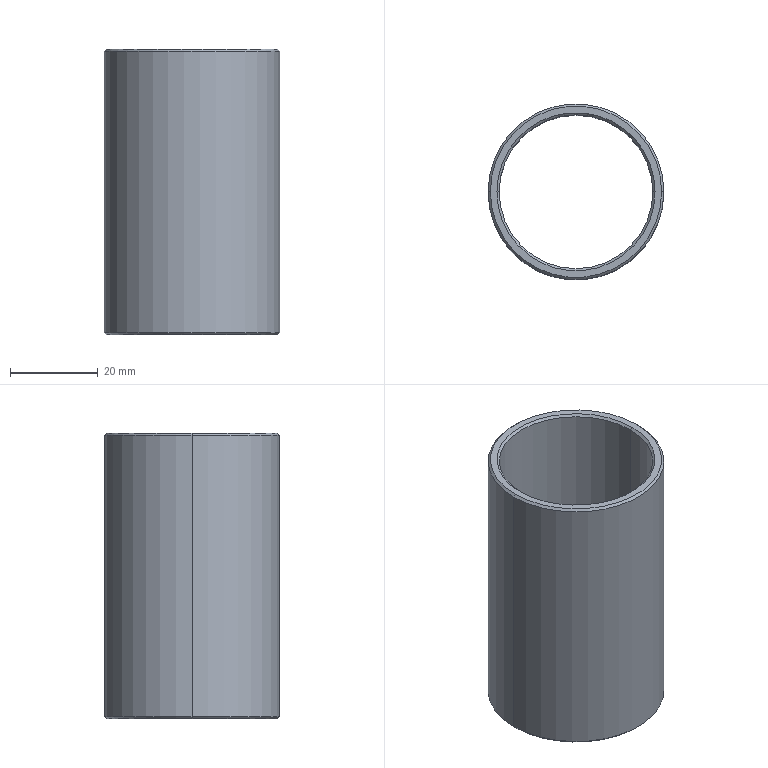Part | STEP file | 40X35X65 oil-free bushing | 1 solid | 14 faces | box 40 x 40 x 65 mm | volume 19085 mm3 | cone 8 | cylinder 4 | plane 2 | commonest cylinder face diameters 35 x2 40 x2
STEP:
#1=CARTESIAN_POINT('',(-17.5,0.,64.5));
#2=VERTEX_POINT('',#1);
#3=CARTESIAN_POINT('',(17.5,0.,64.5));
#4=VERTEX_POINT('',#3);
#5=CARTESIAN_POINT('',(0.,0.,64.5));
#6=DIRECTION('',(0.,0.,1.));
#7=DIRECTION('',(1.,0.,0.));
#8=AXIS2_PLACEMENT_3D('',#5,#6,#7);
#9=CIRCLE('',#8,17.5);
#10=EDGE_CURVE('',#2,#4,#9,.T.);
#11=ORIENTED_EDGE('',*,*,#10,.F.);
#12=CARTESIAN_POINT('',(-18.,0.,65.));
#13=VERTEX_POINT('',#12);
#14=CARTESIAN_POINT('',(-17.5,0.,64.5));
#15=DIRECTION('',(-0.7071,0.,0.7071));
#16=VECTOR('',#15,1000.);
#17=LINE('',#14,#16);
#18=EDGE_CURVE('',#2,#13,#17,.T.);
#19=ORIENTED_EDGE('',*,*,#18,.T.);
#20=CARTESIAN_POINT('',(18.,0.,65.));
#21=VERTEX_POINT('',#20);
#22=CARTESIAN_POINT('',(0.,0.,65.));
#23=DIRECTION('',(0.,0.,-1.));
#24=DIRECTION('',(1.,0.,0.));
#25=AXIS2_PLACEMENT_3D('',#22,#23,#24);
#26=CIRCLE('',#25,18.);
#27=EDGE_CURVE('',#21,#13,#26,.T.);
#28=ORIENTED_EDGE('',*,*,#27,.F.);
#29=CARTESIAN_POINT('',(17.5,0.,64.5));
#30=DIRECTION('',(0.7071,0.,0.7071));
#31=VECTOR('',#30,1000.);
#32=LINE('',#29,#31);
#33=EDGE_CURVE('',#4,#21,#32,.T.);
#34=ORIENTED_EDGE('',*,*,#33,.F.);
#35=EDGE_LOOP('',(#11,#19,#28,#34));
#36=FACE_OUTER_BOUND('',#35,.T.);
#37=CARTESIAN_POINT('',(0.,0.,64.5));
#38=DIRECTION('',(0.,0.,1.));
#39=DIRECTION('',(1.,0.,0.));
#40=AXIS2_PLACEMENT_3D('',#37,#38,#39);
#41=CONICAL_SURFACE('',#40,17.5,0.7854);
#42=ADVANCED_FACE('',(#36),#41,.F.);
#43=CARTESIAN_POINT('',(19.5,0.,65.));
#44=VERTEX_POINT('',#43);
#45=CARTESIAN_POINT('',(-19.5,0.,65.));
#46=VERTEX_POINT('',#45);
#47=CARTESIAN_POINT('',(0.,0.,65.));
#48=DIRECTION('',(0.,0.,1.));
#49=DIRECTION('',(1.,0.,0.));
#50=AXIS2_PLACEMENT_3D('',#47,#48,#49);
#51=CIRCLE('',#50,19.5);
#52=EDGE_CURVE('',#44,#46,#51,.T.);
#53=ORIENTED_EDGE('',*,*,#52,.F.);
#54=CARTESIAN_POINT('',(20.,0.,64.5));
#55=VERTEX_POINT('',#54);
#56=CARTESIAN_POINT('',(19.5,0.,65.));
#57=DIRECTION('',(0.7071,0.,-0.7071));
#58=VECTOR('',#57,1000.);
#59=LINE('',#56,#58);
#60=EDGE_CURVE('',#44,#55,#59,.T.);
#61=ORIENTED_EDGE('',*,*,#60,.T.);
#62=CARTESIAN_POINT('',(-20.,0.,64.5));
#63=VERTEX_POINT('',#62);
#64=CARTESIAN_POINT('',(0.,0.,64.5));
#65=DIRECTION('',(0.,0.,-1.));
#66=DIRECTION('',(1.,0.,0.));
#67=AXIS2_PLACEMENT_3D('',#64,#65,#66);
#68=CIRCLE('',#67,20.);
#69=EDGE_CURVE('',#63,#55,#68,.T.);
#70=ORIENTED_EDGE('',*,*,#69,.F.);
#71=CARTESIAN_POINT('',(-19.5,0.,65.));
#72=DIRECTION('',(-0.7071,0.,-0.7071));
#73=VECTOR('',#72,1000.);
#74=LINE('',#71,#73);
#75=EDGE_CURVE('',#46,#63,#74,.T.);
#76=ORIENTED_EDGE('',*,*,#75,.F.);
#77=EDGE_LOOP('',(#53,#61,#70,#76));
#78=FACE_OUTER_BOUND('',#77,.T.);
#79=CARTESIAN_POINT('',(0.,0.,65.));
#80=DIRECTION('',(0.,0.,-1.));
#81=DIRECTION('',(-1.,0.,0.));
#82=AXIS2_PLACEMENT_3D('',#79,#80,#81);
#83=CONICAL_SURFACE('',#82,19.5,0.7854);
#84=ADVANCED_FACE('',(#78),#83,.T.);
#85=CARTESIAN_POINT('',(-19.5,0.,0.));
#86=VERTEX_POINT('',#85);
#87=CARTESIAN_POINT('',(19.5,0.,0.));
#88=VERTEX_POINT('',#87);
#89=CARTESIAN_POINT('',(0.,0.,0.));
#90=DIRECTION('',(0.,0.,-1.));
#91=DIRECTION('',(1.,0.,0.));
#92=AXIS2_PLACEMENT_3D('',#89,#90,#91);
#93=CIRCLE('',#92,19.5);
#94=EDGE_CURVE('',#86,#88,#93,.T.);
#95=ORIENTED_EDGE('',*,*,#94,.F.);
#96=CARTESIAN_POINT('',(-20.,0.,0.5));
#97=VERTEX_POINT('',#96);
#98=CARTESIAN_POINT('',(-20.,0.,0.5));
#99=DIRECTION('',(-0.7071,0.,0.7071));
#100=VECTOR('',#99,1000.);
#101=LINE('',#98,#100);
#102=EDGE_CURVE('',#86,#97,#101,.T.);
#103=ORIENTED_EDGE('',*,*,#102,.T.);
#104=CARTESIAN_POINT('',(20.,0.,0.5));
#105=VERTEX_POINT('',#104);
#106=CARTESIAN_POINT('',(0.,0.,0.5));
#107=DIRECTION('',(0.,0.,1.));
#108=DIRECTION('',(1.,0.,0.));
#109=AXIS2_PLACEMENT_3D('',#106,#107,#108);
#110=CIRCLE('',#109,20.);
#111=EDGE_CURVE('',#105,#97,#110,.T.);
#112=ORIENTED_EDGE('',*,*,#111,.F.);
#113=CARTESIAN_POINT('',(20.,0.,0.5));
#114=DIRECTION('',(0.7071,0.,0.7071));
#115=VECTOR('',#114,1000.);
#116=LINE('',#113,#115);
#117=EDGE_CURVE('',#88,#105,#116,.T.);
#118=ORIENTED_EDGE('',*,*,#117,.F.);
#119=EDGE_LOOP('',(#95,#103,#112,#118));
#120=FACE_OUTER_BOUND('',#119,.T.);
#121=CARTESIAN_POINT('',(0.,0.,0.5));
#122=DIRECTION('',(0.,0.,1.));
#123=DIRECTION('',(1.,0.,0.));
#124=AXIS2_PLACEMENT_3D('',#121,#122,#123);
#125=CONICAL_SURFACE('',#124,20.,0.7854);
#126=ADVANCED_FACE('',(#120),#125,.T.);
#127=CARTESIAN_POINT('',(17.5,0.,0.5));
#128=VERTEX_POINT('',#127);
#129=CARTESIAN_POINT('',(-17.5,0.,0.5));
#130=VERTEX_POINT('',#129);
#131=CARTESIAN_POINT('',(0.,0.,0.5));
#132=DIRECTION('',(0.,0.,-1.));
#133=DIRECTION('',(1.,0.,0.));
#134=AXIS2_PLACEMENT_3D('',#131,#132,#133);
#135=CIRCLE('',#134,17.5);
#136=EDGE_CURVE('',#128,#130,#135,.T.);
#137=ORIENTED_EDGE('',*,*,#136,.F.);
#138=CARTESIAN_POINT('',(18.,0.,0.));
#139=VERTEX_POINT('',#138);
#140=CARTESIAN_POINT('',(18.,0.,0.));
#141=DIRECTION('',(0.7071,0.,-0.7071));
#142=VECTOR('',#141,1000.);
#143=LINE('',#140,#142);
#144=EDGE_CURVE('',#128,#139,#143,.T.);
#145=ORIENTED_EDGE('',*,*,#144,.T.);
#146=CARTESIAN_POINT('',(-18.,0.,0.));
#147=VERTEX_POINT('',#146);
#148=CARTESIAN_POINT('',(0.,0.,0.));
#149=DIRECTION('',(0.,0.,1.));
#150=DIRECTION('',(1.,0.,0.));
#151=AXIS2_PLACEMENT_3D('',#148,#149,#150);
#152=CIRCLE('',#151,18.);
#153=EDGE_CURVE('',#147,#139,#152,.T.);
#154=ORIENTED_EDGE('',*,*,#153,.F.);
#155=CARTESIAN_POINT('',(-18.,0.,0.));
#156=DIRECTION('',(-0.7071,0.,-0.7071));
#157=VECTOR('',#156,1000.);
#158=LINE('',#155,#157);
#159=EDGE_CURVE('',#130,#147,#158,.T.);
#160=ORIENTED_EDGE('',*,*,#159,.F.);
#161=EDGE_LOOP('',(#137,#145,#154,#160));
#162=FACE_OUTER_BOUND('',#161,.T.);
#163=CARTESIAN_POINT('',(0.,0.,0.));
#164=DIRECTION('',(0.,0.,-1.));
#165=DIRECTION('',(-1.,0.,0.));
#166=AXIS2_PLACEMENT_3D('',#163,#164,#165);
#167=CONICAL_SURFACE('',#166,18.,0.7854);
#168=ADVANCED_FACE('',(#162),#167,.F.);
#169=ORIENTED_EDGE('',*,*,#10,.T.);
#170=CARTESIAN_POINT('',(17.5,0.,65.));
#171=DIRECTION('',(0.,0.,-1.));
#172=VECTOR('',#171,1000.);
#173=LINE('',#170,#172);
#174=EDGE_CURVE('',#4,#128,#173,.T.);
#175=ORIENTED_EDGE('',*,*,#174,.T.);
#176=ORIENTED_EDGE('',*,*,#136,.T.);
#177=CARTESIAN_POINT('',(-17.5,0.,65.));
#178=DIRECTION('',(0.,0.,-1.));
#179=VECTOR('',#178,1000.);
#180=LINE('',#177,#179);
#181=EDGE_CURVE('',#2,#130,#180,.T.);
#182=ORIENTED_EDGE('',*,*,#181,.F.);
#183=EDGE_LOOP('',(#169,#175,#176,#182));
#184=FACE_OUTER_BOUND('',#183,.T.);
#185=CARTESIAN_POINT('',(0.,0.,65.));
#186=DIRECTION('',(0.,0.,-1.));
#187=DIRECTION('',(-1.,0.,0.));
#188=AXIS2_PLACEMENT_3D('',#185,#186,#187);
#189=CYLINDRICAL_SURFACE('',#188,17.5);
#190=ADVANCED_FACE('',(#184),#189,.F.);
#191=ORIENTED_EDGE('',*,*,#69,.T.);
#192=CARTESIAN_POINT('',(20.,0.,65.));
#193=DIRECTION('',(0.,0.,-1.));
#194=VECTOR('',#193,1000.);
#195=LINE('',#192,#194);
#196=EDGE_CURVE('',#55,#105,#195,.T.);
#197=ORIENTED_EDGE('',*,*,#196,.T.);
#198=ORIENTED_EDGE('',*,*,#111,.T.);
#199=CARTESIAN_POINT('',(-20.,0.,65.));
#200=DIRECTION('',(0.,0.,-1.));
#201=VECTOR('',#200,1000.);
#202=LINE('',#199,#201);
#203=EDGE_CURVE('',#63,#97,#202,.T.);
#204=ORIENTED_EDGE('',*,*,#203,.F.);
#205=EDGE_LOOP('',(#191,#197,#198,#204));
#206=FACE_OUTER_BOUND('',#205,.T.);
#207=CARTESIAN_POINT('',(0.,0.,65.));
#208=DIRECTION('',(0.,0.,-1.));
#209=DIRECTION('',(-1.,0.,0.));
#210=AXIS2_PLACEMENT_3D('',#207,#208,#209);
#211=CYLINDRICAL_SURFACE('',#210,20.);
#212=ADVANCED_FACE('',(#206),#211,.T.);
#213=CARTESIAN_POINT('',(0.,0.,65.));
#214=DIRECTION('',(0.,0.,1.));
#215=DIRECTION('',(1.,0.,0.));
#216=AXIS2_PLACEMENT_3D('',#213,#214,#215);
#217=CIRCLE('',#216,19.5);
#218=EDGE_CURVE('',#46,#44,#217,.T.);
#219=ORIENTED_EDGE('',*,*,#218,.T.);
#220=ORIENTED_EDGE('',*,*,#52,.T.);
#221=EDGE_LOOP('',(#219,#220));
#222=FACE_OUTER_BOUND('',#221,.T.);
#223=ORIENTED_EDGE('',*,*,#27,.T.);
#224=CARTESIAN_POINT('',(0.,0.,65.));
#225=DIRECTION('',(0.,0.,-1.));
#226=DIRECTION('',(1.,0.,0.));
#227=AXIS2_PLACEMENT_3D('',#224,#225,#226);
#228=CIRCLE('',#227,18.);
#229=EDGE_CURVE('',#13,#21,#228,.T.);
#230=ORIENTED_EDGE('',*,*,#229,.T.);
#231=EDGE_LOOP('',(#223,#230));
#232=FACE_BOUND('',#231,.T.);
#233=CARTESIAN_POINT('',(0.,0.,65.));
#234=DIRECTION('',(0.,0.,1.));
#235=DIRECTION('',(1.,0.,0.));
#236=AXIS2_PLACEMENT_3D('',#233,#234,#235);
#237=PLANE('',#236);
#238=ADVANCED_FACE('',(#222,#232),#237,.T.);
#239=ORIENTED_EDGE('',*,*,#153,.T.);
#240=CARTESIAN_POINT('',(0.,0.,0.));
#241=DIRECTION('',(0.,0.,1.));
#242=DIRECTION('',(1.,0.,0.));
#243=AXIS2_PLACEMENT_3D('',#240,#241,#242);
#244=CIRCLE('',#243,18.);
#245=EDGE_CURVE('',#139,#147,#244,.T.);
#246=ORIENTED_EDGE('',*,*,#245,.T.);
#247=EDGE_LOOP('',(#239,#246));
#248=FACE_BOUND('',#247,.T.);
#249=CARTESIAN_POINT('',(0.,0.,0.));
#250=DIRECTION('',(0.,0.,-1.));
#251=DIRECTION('',(1.,0.,0.));
#252=AXIS2_PLACEMENT_3D('',#249,#250,#251);
#253=CIRCLE('',#252,19.5);
#254=EDGE_CURVE('',#88,#86,#253,.T.);
#255=ORIENTED_EDGE('',*,*,#254,.T.);
#256=ORIENTED_EDGE('',*,*,#94,.T.);
#257=EDGE_LOOP('',(#255,#256));
#258=FACE_OUTER_BOUND('',#257,.T.);
#259=CARTESIAN_POINT('',(0.,0.,0.));
#260=DIRECTION('',(0.,0.,1.));
#261=DIRECTION('',(1.,0.,0.));
#262=AXIS2_PLACEMENT_3D('',#259,#260,#261);
#263=PLANE('',#262);
#264=ADVANCED_FACE('',(#248,#258),#263,.F.);
#265=ORIENTED_EDGE('',*,*,#196,.F.);
#266=CARTESIAN_POINT('',(0.,0.,64.5));
#267=DIRECTION('',(0.,0.,-1.));
#268=DIRECTION('',(1.,0.,0.));
#269=AXIS2_PLACEMENT_3D('',#266,#267,#268);
#270=CIRCLE('',#269,20.);
#271=EDGE_CURVE('',#55,#63,#270,.T.);
#272=ORIENTED_EDGE('',*,*,#271,.T.);
#273=ORIENTED_EDGE('',*,*,#203,.T.);
#274=CARTESIAN_POINT('',(0.,0.,0.5));
#275=DIRECTION('',(0.,0.,1.));
#276=DIRECTION('',(1.,0.,0.));
#277=AXIS2_PLACEMENT_3D('',#274,#275,#276);
#278=CIRCLE('',#277,20.);
#279=EDGE_CURVE('',#97,#105,#278,.T.);
#280=ORIENTED_EDGE('',*,*,#279,.T.);
#281=EDGE_LOOP('',(#265,#272,#273,#280));
#282=FACE_OUTER_BOUND('',#281,.T.);
#283=CARTESIAN_POINT('',(0.,0.,65.));
#284=DIRECTION('',(0.,0.,-1.));
#285=DIRECTION('',(-1.,0.,0.));
#286=AXIS2_PLACEMENT_3D('',#283,#284,#285);
#287=CYLINDRICAL_SURFACE('',#286,20.);
#288=ADVANCED_FACE('',(#282),#287,.T.);
#289=ORIENTED_EDGE('',*,*,#174,.F.);
#290=CARTESIAN_POINT('',(0.,0.,64.5));
#291=DIRECTION('',(0.,0.,1.));
#292=DIRECTION('',(1.,0.,0.));
#293=AXIS2_PLACEMENT_3D('',#290,#291,#292);
#294=CIRCLE('',#293,17.5);
#295=EDGE_CURVE('',#4,#2,#294,.T.);
#296=ORIENTED_EDGE('',*,*,#295,.T.);
#297=ORIENTED_EDGE('',*,*,#181,.T.);
#298=CARTESIAN_POINT('',(0.,0.,0.5));
#299=DIRECTION('',(0.,0.,-1.));
#300=DIRECTION('',(1.,0.,0.));
#301=AXIS2_PLACEMENT_3D('',#298,#299,#300);
#302=CIRCLE('',#301,17.5);
#303=EDGE_CURVE('',#130,#128,#302,.T.);
#304=ORIENTED_EDGE('',*,*,#303,.T.);
#305=EDGE_LOOP('',(#289,#296,#297,#304));
#306=FACE_OUTER_BOUND('',#305,.T.);
#307=CARTESIAN_POINT('',(0.,0.,65.));
#308=DIRECTION('',(0.,0.,-1.));
#309=DIRECTION('',(-1.,0.,0.));
#310=AXIS2_PLACEMENT_3D('',#307,#308,#309);
#311=CYLINDRICAL_SURFACE('',#310,17.5);
#312=ADVANCED_FACE('',(#306),#311,.F.);
#313=ORIENTED_EDGE('',*,*,#144,.F.);
#314=ORIENTED_EDGE('',*,*,#303,.F.);
#315=ORIENTED_EDGE('',*,*,#159,.T.);
#316=ORIENTED_EDGE('',*,*,#245,.F.);
#317=EDGE_LOOP('',(#313,#314,#315,#316));
#318=FACE_OUTER_BOUND('',#317,.T.);
#319=CARTESIAN_POINT('',(0.,0.,0.));
#320=DIRECTION('',(0.,0.,-1.));
#321=DIRECTION('',(-1.,0.,0.));
#322=AXIS2_PLACEMENT_3D('',#319,#320,#321);
#323=CONICAL_SURFACE('',#322,18.,0.7854);
#324=ADVANCED_FACE('',(#318),#323,.F.);
#325=ORIENTED_EDGE('',*,*,#102,.F.);
#326=ORIENTED_EDGE('',*,*,#254,.F.);
#327=ORIENTED_EDGE('',*,*,#117,.T.);
#328=ORIENTED_EDGE('',*,*,#279,.F.);
#329=EDGE_LOOP('',(#325,#326,#327,#328));
#330=FACE_OUTER_BOUND('',#329,.T.);
#331=CARTESIAN_POINT('',(0.,0.,0.5));
#332=DIRECTION('',(0.,0.,1.));
#333=DIRECTION('',(1.,0.,0.));
#334=AXIS2_PLACEMENT_3D('',#331,#332,#333);
#335=CONICAL_SURFACE('',#334,20.,0.7854);
#336=ADVANCED_FACE('',(#330),#335,.T.);
#337=ORIENTED_EDGE('',*,*,#60,.F.);
#338=ORIENTED_EDGE('',*,*,#218,.F.);
#339=ORIENTED_EDGE('',*,*,#75,.T.);
#340=ORIENTED_EDGE('',*,*,#271,.F.);
#341=EDGE_LOOP('',(#337,#338,#339,#340));
#342=FACE_OUTER_BOUND('',#341,.T.);
#343=CARTESIAN_POINT('',(0.,0.,65.));
#344=DIRECTION('',(0.,0.,-1.));
#345=DIRECTION('',(-1.,0.,0.));
#346=AXIS2_PLACEMENT_3D('',#343,#344,#345);
#347=CONICAL_SURFACE('',#346,19.5,0.7854);
#348=ADVANCED_FACE('',(#342),#347,.T.);
#349=ORIENTED_EDGE('',*,*,#18,.F.);
#350=ORIENTED_EDGE('',*,*,#295,.F.);
#351=ORIENTED_EDGE('',*,*,#33,.T.);
#352=ORIENTED_EDGE('',*,*,#229,.F.);
#353=EDGE_LOOP('',(#349,#350,#351,#352));
#354=FACE_OUTER_BOUND('',#353,.T.);
#355=CARTESIAN_POINT('',(0.,0.,64.5));
#356=DIRECTION('',(0.,0.,1.));
#357=DIRECTION('',(1.,0.,0.));
#358=AXIS2_PLACEMENT_3D('',#355,#356,#357);
#359=CONICAL_SURFACE('',#358,17.5,0.7854);
#360=ADVANCED_FACE('',(#354),#359,.F.);
#361=CLOSED_SHELL('',(#42,#84,#126,#168,#190,#212,#238,#264,#288,#312,#324,#336,#348,#360));
#362=MANIFOLD_SOLID_BREP('',#361);
#363=CARTESIAN_POINT('',(0.,0.,0.));
#364=DIRECTION('',(0.,0.,1.));
#365=DIRECTION('',(1.,0.,0.));
#366=AXIS2_PLACEMENT_3D('',#363,#364,#365);
#367=(LENGTH_UNIT()NAMED_UNIT(*)SI_UNIT(.MILLI.,.METRE.));
#368=UNCERTAINTY_MEASURE_WITH_UNIT(LENGTH_MEASURE(0.00001),#367,'','');
#369=(NAMED_UNIT(*)PLANE_ANGLE_UNIT()SI_UNIT($,.RADIAN.));
#370=(NAMED_UNIT(*)SI_UNIT($,.STERADIAN.)SOLID_ANGLE_UNIT());
#371=(GEOMETRIC_REPRESENTATION_CONTEXT(3)GLOBAL_UNCERTAINTY_ASSIGNED_CONTEXT((#368))GLOBAL_UNIT_ASSIGNED_CONTEXT((#367,#369,#370))REPRESENTATION_CONTEXT('',''));
#372=ADVANCED_BREP_SHAPE_REPRESENTATION('',(#362,#366),#371);